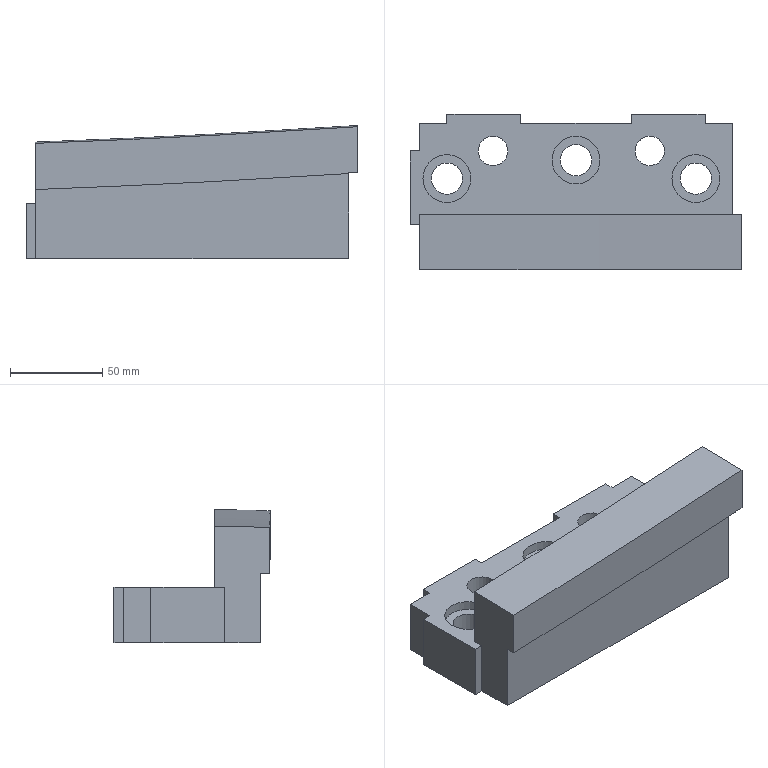Part | NX | features solid 2 | 1 solid | 35 faces | box 180 x 84.614 x 72.162 mm | volume 542810 mm3 | plane 22 | cylinder 8 | spline 5 | commonest cylinder face diameters 17 x3 26 x3 16 x2
STEP:
#1=CARTESIAN_POINT('',(526.5,240.,-40.));
#2=VERTEX_POINT('',#1);
#3=CARTESIAN_POINT('',(535.,240.,-40.));
#4=DIRECTION('',(0.,0.,-1.));
#5=DIRECTION('',(-1.,0.,0.));
#6=AXIS2_PLACEMENT_3D('',#3,#4,#5);
#7=CIRCLE('',#6,8.5);
#8=EDGE_CURVE('',#2,#2,#7,.T.);
#9=ORIENTED_EDGE('',*,*,#8,.F.);
#10=EDGE_LOOP('',(#9));
#11=FACE_BOUND('',#10,.T.);
#12=CARTESIAN_POINT('',(461.5,250.,-40.));
#13=VERTEX_POINT('',#12);
#14=CARTESIAN_POINT('',(470.,250.,-40.));
#15=DIRECTION('',(0.,0.,-1.));
#16=DIRECTION('',(-1.,0.,0.));
#17=AXIS2_PLACEMENT_3D('',#14,#15,#16);
#18=CIRCLE('',#17,8.5);
#19=EDGE_CURVE('',#13,#13,#18,.T.);
#20=ORIENTED_EDGE('',*,*,#19,.F.);
#21=EDGE_LOOP('',(#20));
#22=FACE_BOUND('',#21,.T.);
#23=CARTESIAN_POINT('',(391.5,240.,-40.));
#24=VERTEX_POINT('',#23);
#25=CARTESIAN_POINT('',(400.,240.,-40.));
#26=DIRECTION('',(0.,0.,-1.));
#27=DIRECTION('',(-1.,0.,0.));
#28=AXIS2_PLACEMENT_3D('',#25,#26,#27);
#29=CIRCLE('',#28,8.5);
#30=EDGE_CURVE('',#24,#24,#29,.T.);
#31=ORIENTED_EDGE('',*,*,#30,.F.);
#32=EDGE_LOOP('',(#31));
#33=FACE_BOUND('',#32,.T.);
#34=CARTESIAN_POINT('',(502.,255.,-40.));
#35=VERTEX_POINT('',#34);
#36=CARTESIAN_POINT('',(510.,255.,-40.));
#37=DIRECTION('',(0.,0.,-1.));
#38=DIRECTION('',(-1.,0.,0.));
#39=AXIS2_PLACEMENT_3D('',#36,#37,#38);
#40=CIRCLE('',#39,8.);
#41=EDGE_CURVE('',#35,#35,#40,.F.);
#42=ORIENTED_EDGE('',*,*,#41,.T.);
#43=EDGE_LOOP('',(#42));
#44=FACE_BOUND('',#43,.T.);
#45=CARTESIAN_POINT('',(385.,270.,-40.));
#46=VERTEX_POINT('',#45);
#47=CARTESIAN_POINT('',(385.,255.,-40.));
#48=VERTEX_POINT('',#47);
#49=CARTESIAN_POINT('',(385.,62.718,-40.));
#50=DIRECTION('',(0.,-1.,0.));
#51=VECTOR('',#50,1000.);
#52=LINE('',#49,#51);
#53=EDGE_CURVE('',#46,#48,#52,.T.);
#54=ORIENTED_EDGE('',*,*,#53,.F.);
#55=CARTESIAN_POINT('',(400.,270.,-40.));
#56=VERTEX_POINT('',#55);
#57=CARTESIAN_POINT('',(660.,270.,-40.));
#58=DIRECTION('',(1.,0.,0.));
#59=VECTOR('',#58,1000.);
#60=LINE('',#57,#59);
#61=EDGE_CURVE('',#56,#46,#60,.F.);
#62=ORIENTED_EDGE('',*,*,#61,.F.);
#63=CARTESIAN_POINT('',(400.,275.,-40.));
#64=VERTEX_POINT('',#63);
#65=CARTESIAN_POINT('',(400.,270.,-40.));
#66=DIRECTION('',(0.,-1.,0.));
#67=VECTOR('',#66,1000.);
#68=LINE('',#65,#67);
#69=EDGE_CURVE('',#56,#64,#68,.F.);
#70=ORIENTED_EDGE('',*,*,#69,.T.);
#71=CARTESIAN_POINT('',(440.,275.,-40.));
#72=VERTEX_POINT('',#71);
#73=CARTESIAN_POINT('',(440.,275.,-40.));
#74=DIRECTION('',(1.,0.,0.));
#75=VECTOR('',#74,1000.);
#76=LINE('',#73,#75);
#77=EDGE_CURVE('',#72,#64,#76,.F.);
#78=ORIENTED_EDGE('',*,*,#77,.F.);
#79=CARTESIAN_POINT('',(440.,270.,-40.));
#80=VERTEX_POINT('',#79);
#81=CARTESIAN_POINT('',(440.,270.,-40.));
#82=DIRECTION('',(0.,-1.,0.));
#83=VECTOR('',#82,1000.);
#84=LINE('',#81,#83);
#85=EDGE_CURVE('',#80,#72,#84,.F.);
#86=ORIENTED_EDGE('',*,*,#85,.F.);
#87=CARTESIAN_POINT('',(500.,270.,-40.));
#88=VERTEX_POINT('',#87);
#89=CARTESIAN_POINT('',(660.,270.,-40.));
#90=DIRECTION('',(1.,0.,0.));
#91=VECTOR('',#90,1000.);
#92=LINE('',#89,#91);
#93=EDGE_CURVE('',#88,#80,#92,.F.);
#94=ORIENTED_EDGE('',*,*,#93,.F.);
#95=CARTESIAN_POINT('',(500.,275.,-40.));
#96=VERTEX_POINT('',#95);
#97=CARTESIAN_POINT('',(500.,270.,-40.));
#98=DIRECTION('',(0.,-1.,0.));
#99=VECTOR('',#98,1000.);
#100=LINE('',#97,#99);
#101=EDGE_CURVE('',#88,#96,#100,.F.);
#102=ORIENTED_EDGE('',*,*,#101,.T.);
#103=CARTESIAN_POINT('',(540.,275.,-40.));
#104=VERTEX_POINT('',#103);
#105=CARTESIAN_POINT('',(540.,275.,-40.));
#106=DIRECTION('',(1.,0.,0.));
#107=VECTOR('',#106,1000.);
#108=LINE('',#105,#107);
#109=EDGE_CURVE('',#104,#96,#108,.F.);
#110=ORIENTED_EDGE('',*,*,#109,.F.);
#111=CARTESIAN_POINT('',(540.,270.,-40.));
#112=VERTEX_POINT('',#111);
#113=CARTESIAN_POINT('',(540.,270.,-40.));
#114=DIRECTION('',(0.,-1.,0.));
#115=VECTOR('',#114,1000.);
#116=LINE('',#113,#115);
#117=EDGE_CURVE('',#112,#104,#116,.F.);
#118=ORIENTED_EDGE('',*,*,#117,.F.);
#119=CARTESIAN_POINT('',(555.,270.,-40.));
#120=VERTEX_POINT('',#119);
#121=CARTESIAN_POINT('',(660.,270.,-40.));
#122=DIRECTION('',(1.,0.,0.));
#123=VECTOR('',#122,1000.);
#124=LINE('',#121,#123);
#125=EDGE_CURVE('',#120,#112,#124,.F.);
#126=ORIENTED_EDGE('',*,*,#125,.F.);
#127=CARTESIAN_POINT('',(555.,195.38,-40.));
#128=VERTEX_POINT('',#127);
#129=CARTESIAN_POINT('',(555.,62.718,-40.));
#130=DIRECTION('',(0.,1.,0.));
#131=VECTOR('',#130,1000.);
#132=LINE('',#129,#131);
#133=EDGE_CURVE('',#128,#120,#132,.T.);
#134=ORIENTED_EDGE('',*,*,#133,.F.);
#135=CARTESIAN_POINT('',(385.,195.487,-40.));
#136=VERTEX_POINT('',#135);
#137=CARTESIAN_POINT('',(385.,195.487,-40.));
#138=CARTESIAN_POINT('',(413.333,195.462,-40.));
#139=CARTESIAN_POINT('',(470.,195.441,-40.));
#140=CARTESIAN_POINT('',(526.667,195.352,-40.));
#141=CARTESIAN_POINT('',(555.,195.38,-40.));
#142=B_SPLINE_CURVE_WITH_KNOTS('',3,(#137,#138,#139,#140,#141),.UNSPECIFIED.,.F.,.F.,(4,1,4),(0.1223,0.2065,0.2908),.UNSPECIFIED.);
#143=EDGE_CURVE('',#136,#128,#142,.T.);
#144=ORIENTED_EDGE('',*,*,#143,.F.);
#145=CARTESIAN_POINT('',(385.,215.,-40.));
#146=VERTEX_POINT('',#145);
#147=CARTESIAN_POINT('',(385.,62.718,-40.));
#148=DIRECTION('',(0.,-1.,0.));
#149=VECTOR('',#148,1000.);
#150=LINE('',#147,#149);
#151=EDGE_CURVE('',#146,#136,#150,.T.);
#152=ORIENTED_EDGE('',*,*,#151,.F.);
#153=CARTESIAN_POINT('',(380.,215.,-40.));
#154=VERTEX_POINT('',#153);
#155=CARTESIAN_POINT('',(385.,215.,-40.));
#156=DIRECTION('',(1.,0.,0.));
#157=VECTOR('',#156,1000.);
#158=LINE('',#155,#157);
#159=EDGE_CURVE('',#146,#154,#158,.F.);
#160=ORIENTED_EDGE('',*,*,#159,.T.);
#161=CARTESIAN_POINT('',(380.,255.,-40.));
#162=VERTEX_POINT('',#161);
#163=CARTESIAN_POINT('',(380.,270.,-40.));
#164=DIRECTION('',(0.,1.,0.));
#165=VECTOR('',#164,1000.);
#166=LINE('',#163,#165);
#167=EDGE_CURVE('',#154,#162,#166,.T.);
#168=ORIENTED_EDGE('',*,*,#167,.T.);
#169=CARTESIAN_POINT('',(385.,255.,-40.));
#170=DIRECTION('',(1.,0.,0.));
#171=VECTOR('',#170,1000.);
#172=LINE('',#169,#171);
#173=EDGE_CURVE('',#48,#162,#172,.F.);
#174=ORIENTED_EDGE('',*,*,#173,.F.);
#175=EDGE_LOOP('',(#54,#62,#70,#78,#86,#94,#102,#110,#118,#126,#134,#144,#152,#160,#168,#174));
#176=FACE_BOUND('',#175,.T.);
#177=CARTESIAN_POINT('',(417.,255.,-40.));
#178=VERTEX_POINT('',#177);
#179=CARTESIAN_POINT('',(425.,255.,-40.));
#180=DIRECTION('',(0.,0.,-1.));
#181=DIRECTION('',(-1.,0.,0.));
#182=AXIS2_PLACEMENT_3D('',#179,#180,#181);
#183=CIRCLE('',#182,8.);
#184=EDGE_CURVE('',#178,#178,#183,.F.);
#185=ORIENTED_EDGE('',*,*,#184,.T.);
#186=EDGE_LOOP('',(#185));
#187=FACE_BOUND('',#186,.T.);
#188=CARTESIAN_POINT('',(248.595,62.718,-40.));
#189=DIRECTION('',(0.,0.,-1.));
#190=DIRECTION('',(1.,0.,0.));
#191=AXIS2_PLACEMENT_3D('',#188,#189,#190);
#192=PLANE('',#191);
#193=ADVANCED_FACE('',(#11,#22,#33,#44,#176,#187),#192,.T.);
#194=CARTESIAN_POINT('',(522.,240.,-10.));
#195=VERTEX_POINT('',#194);
#196=CARTESIAN_POINT('',(535.,240.,-10.));
#197=DIRECTION('',(0.,0.,-1.));
#198=DIRECTION('',(-1.,0.,0.));
#199=AXIS2_PLACEMENT_3D('',#196,#197,#198);
#200=CIRCLE('',#199,13.);
#201=EDGE_CURVE('',#195,#195,#200,.T.);
#202=ORIENTED_EDGE('',*,*,#201,.T.);
#203=EDGE_LOOP('',(#202));
#204=FACE_BOUND('',#203,.T.);
#205=CARTESIAN_POINT('',(457.,250.,-10.));
#206=VERTEX_POINT('',#205);
#207=CARTESIAN_POINT('',(470.,250.,-10.));
#208=DIRECTION('',(0.,0.,-1.));
#209=DIRECTION('',(-1.,0.,0.));
#210=AXIS2_PLACEMENT_3D('',#207,#208,#209);
#211=CIRCLE('',#210,13.);
#212=EDGE_CURVE('',#206,#206,#211,.T.);
#213=ORIENTED_EDGE('',*,*,#212,.T.);
#214=EDGE_LOOP('',(#213));
#215=FACE_BOUND('',#214,.T.);
#216=CARTESIAN_POINT('',(387.,240.,-10.));
#217=VERTEX_POINT('',#216);
#218=CARTESIAN_POINT('',(400.,240.,-10.));
#219=DIRECTION('',(0.,0.,-1.));
#220=DIRECTION('',(-1.,0.,0.));
#221=AXIS2_PLACEMENT_3D('',#218,#219,#220);
#222=CIRCLE('',#221,13.);
#223=EDGE_CURVE('',#217,#217,#222,.T.);
#224=ORIENTED_EDGE('',*,*,#223,.T.);
#225=EDGE_LOOP('',(#224));
#226=FACE_BOUND('',#225,.T.);
#227=CARTESIAN_POINT('',(502.,255.,-10.));
#228=VERTEX_POINT('',#227);
#229=CARTESIAN_POINT('',(510.,255.,-10.));
#230=DIRECTION('',(0.,0.,-1.));
#231=DIRECTION('',(-1.,0.,0.));
#232=AXIS2_PLACEMENT_3D('',#229,#230,#231);
#233=CIRCLE('',#232,8.);
#234=EDGE_CURVE('',#228,#228,#233,.F.);
#235=ORIENTED_EDGE('',*,*,#234,.F.);
#236=EDGE_LOOP('',(#235));
#237=FACE_BOUND('',#236,.T.);
#238=CARTESIAN_POINT('',(555.,270.,-10.));
#239=VERTEX_POINT('',#238);
#240=CARTESIAN_POINT('',(540.,270.,-10.));
#241=VERTEX_POINT('',#240);
#242=CARTESIAN_POINT('',(660.,270.,-10.));
#243=DIRECTION('',(-1.,0.,0.));
#244=VECTOR('',#243,1000.);
#245=LINE('',#242,#244);
#246=EDGE_CURVE('',#239,#241,#245,.T.);
#247=ORIENTED_EDGE('',*,*,#246,.T.);
#248=CARTESIAN_POINT('',(540.,275.,-10.));
#249=VERTEX_POINT('',#248);
#250=CARTESIAN_POINT('',(540.,270.,-10.));
#251=DIRECTION('',(0.,-1.,0.));
#252=VECTOR('',#251,1000.);
#253=LINE('',#250,#252);
#254=EDGE_CURVE('',#241,#249,#253,.F.);
#255=ORIENTED_EDGE('',*,*,#254,.T.);
#256=CARTESIAN_POINT('',(500.,275.,-10.));
#257=VERTEX_POINT('',#256);
#258=CARTESIAN_POINT('',(540.,275.,-10.));
#259=DIRECTION('',(1.,0.,0.));
#260=VECTOR('',#259,1000.);
#261=LINE('',#258,#260);
#262=EDGE_CURVE('',#249,#257,#261,.F.);
#263=ORIENTED_EDGE('',*,*,#262,.T.);
#264=CARTESIAN_POINT('',(500.,270.,-10.));
#265=VERTEX_POINT('',#264);
#266=CARTESIAN_POINT('',(500.,270.,-10.));
#267=DIRECTION('',(0.,-1.,0.));
#268=VECTOR('',#267,1000.);
#269=LINE('',#266,#268);
#270=EDGE_CURVE('',#265,#257,#269,.F.);
#271=ORIENTED_EDGE('',*,*,#270,.F.);
#272=CARTESIAN_POINT('',(440.,270.,-10.));
#273=VERTEX_POINT('',#272);
#274=CARTESIAN_POINT('',(660.,270.,-10.));
#275=DIRECTION('',(-1.,0.,0.));
#276=VECTOR('',#275,1000.);
#277=LINE('',#274,#276);
#278=EDGE_CURVE('',#265,#273,#277,.T.);
#279=ORIENTED_EDGE('',*,*,#278,.T.);
#280=CARTESIAN_POINT('',(440.,275.,-10.));
#281=VERTEX_POINT('',#280);
#282=CARTESIAN_POINT('',(440.,270.,-10.));
#283=DIRECTION('',(0.,-1.,0.));
#284=VECTOR('',#283,1000.);
#285=LINE('',#282,#284);
#286=EDGE_CURVE('',#273,#281,#285,.F.);
#287=ORIENTED_EDGE('',*,*,#286,.T.);
#288=CARTESIAN_POINT('',(400.,275.,-10.));
#289=VERTEX_POINT('',#288);
#290=CARTESIAN_POINT('',(440.,275.,-10.));
#291=DIRECTION('',(1.,0.,0.));
#292=VECTOR('',#291,1000.);
#293=LINE('',#290,#292);
#294=EDGE_CURVE('',#281,#289,#293,.F.);
#295=ORIENTED_EDGE('',*,*,#294,.T.);
#296=CARTESIAN_POINT('',(400.,270.,-10.));
#297=VERTEX_POINT('',#296);
#298=CARTESIAN_POINT('',(400.,270.,-10.));
#299=DIRECTION('',(0.,-1.,0.));
#300=VECTOR('',#299,1000.);
#301=LINE('',#298,#300);
#302=EDGE_CURVE('',#297,#289,#301,.F.);
#303=ORIENTED_EDGE('',*,*,#302,.F.);
#304=CARTESIAN_POINT('',(385.,270.,-10.));
#305=VERTEX_POINT('',#304);
#306=CARTESIAN_POINT('',(660.,270.,-10.));
#307=DIRECTION('',(-1.,0.,0.));
#308=VECTOR('',#307,1000.);
#309=LINE('',#306,#308);
#310=EDGE_CURVE('',#297,#305,#309,.T.);
#311=ORIENTED_EDGE('',*,*,#310,.T.);
#312=CARTESIAN_POINT('',(385.,255.,-10.));
#313=VERTEX_POINT('',#312);
#314=CARTESIAN_POINT('',(385.,270.,-10.));
#315=DIRECTION('',(0.,-1.,0.));
#316=VECTOR('',#315,1000.);
#317=LINE('',#314,#316);
#318=EDGE_CURVE('',#305,#313,#317,.T.);
#319=ORIENTED_EDGE('',*,*,#318,.T.);
#320=CARTESIAN_POINT('',(380.,255.,-10.));
#321=VERTEX_POINT('',#320);
#322=CARTESIAN_POINT('',(385.,255.,-10.));
#323=DIRECTION('',(1.,0.,0.));
#324=VECTOR('',#323,1000.);
#325=LINE('',#322,#324);
#326=EDGE_CURVE('',#313,#321,#325,.F.);
#327=ORIENTED_EDGE('',*,*,#326,.T.);
#328=CARTESIAN_POINT('',(380.,215.,-10.));
#329=VERTEX_POINT('',#328);
#330=CARTESIAN_POINT('',(380.,270.,-10.));
#331=DIRECTION('',(0.,1.,0.));
#332=VECTOR('',#331,1000.);
#333=LINE('',#330,#332);
#334=EDGE_CURVE('',#329,#321,#333,.T.);
#335=ORIENTED_EDGE('',*,*,#334,.F.);
#336=CARTESIAN_POINT('',(385.,215.,-10.));
#337=VERTEX_POINT('',#336);
#338=CARTESIAN_POINT('',(385.,215.,-10.));
#339=DIRECTION('',(1.,0.,0.));
#340=VECTOR('',#339,1000.);
#341=LINE('',#338,#340);
#342=EDGE_CURVE('',#337,#329,#341,.F.);
#343=ORIENTED_EDGE('',*,*,#342,.F.);
#344=CARTESIAN_POINT('',(385.,220.484,-10.));
#345=VERTEX_POINT('',#344);
#346=CARTESIAN_POINT('',(385.,270.,-10.));
#347=DIRECTION('',(0.,1.,0.));
#348=VECTOR('',#347,1000.);
#349=LINE('',#346,#348);
#350=EDGE_CURVE('',#337,#345,#349,.T.);
#351=ORIENTED_EDGE('',*,*,#350,.T.);
#352=CARTESIAN_POINT('',(555.,220.387,-10.));
#353=VERTEX_POINT('',#352);
#354=CARTESIAN_POINT('',(560.,220.386,-10.));
#355=CARTESIAN_POINT('',(526.442,220.392,-10.));
#356=CARTESIAN_POINT('',(476.105,220.419,-10.));
#357=CARTESIAN_POINT('',(408.97,220.463,-10.));
#358=CARTESIAN_POINT('',(366.895,220.496,-10.));
#359=CARTESIAN_POINT('',(333.741,220.565,-10.));
#360=CARTESIAN_POINT('',(314.827,220.599,-10.));
#361=CARTESIAN_POINT('',(301.695,220.599,-10.));
#362=CARTESIAN_POINT('',(297.997,220.637,-10.));
#363=CARTESIAN_POINT('',(290.161,220.611,-10.));
#364=CARTESIAN_POINT('',(281.479,219.228,-10.));
#365=CARTESIAN_POINT('',(272.181,215.568,-10.));
#366=CARTESIAN_POINT('',(264.352,210.189,-10.));
#367=CARTESIAN_POINT('',(257.821,203.431,-10.));
#368=CARTESIAN_POINT('',(253.634,196.762,-10.));
#369=CARTESIAN_POINT('',(251.086,190.582,-10.));
#370=CARTESIAN_POINT('',(249.212,184.171,-10.));
#371=CARTESIAN_POINT('',(248.528,177.262,-10.));
#372=CARTESIAN_POINT('',(248.548,172.265,-10.));
#373=CARTESIAN_POINT('',(248.587,169.669,-10.));
#374=CARTESIAN_POINT('',(248.59,166.626,-10.));
#375=CARTESIAN_POINT('',(248.575,155.998,-10.));
#376=CARTESIAN_POINT('',(248.59,138.236,-10.));
#377=CARTESIAN_POINT('',(248.599,104.71,-10.));
#378=CARTESIAN_POINT('',(248.592,45.941,-10.));
#379=CARTESIAN_POINT('',(248.598,-12.772,-10.));
#380=CARTESIAN_POINT('',(248.605,-63.152,-10.));
#381=CARTESIAN_POINT('',(248.59,-84.03,-10.));
#382=CARTESIAN_POINT('',(248.581,-100.973,-10.));
#383=CARTESIAN_POINT('',(248.614,-110.39,-10.));
#384=CARTESIAN_POINT('',(248.565,-116.228,-10.));
#385=CARTESIAN_POINT('',(248.487,-119.918,-10.));
#386=CARTESIAN_POINT('',(248.926,-126.9,-10.));
#387=CARTESIAN_POINT('',(250.444,-133.072,-10.));
#388=CARTESIAN_POINT('',(252.598,-139.093,-10.));
#389=CARTESIAN_POINT('',(256.391,-145.942,-10.));
#390=CARTESIAN_POINT('',(262.559,-153.127,-10.));
#391=CARTESIAN_POINT('',(270.075,-158.887,-10.));
#392=CARTESIAN_POINT('',(277.474,-162.344,-10.));
#393=CARTESIAN_POINT('',(283.712,-164.068,-10.));
#394=CARTESIAN_POINT('',(289.455,-165.043,-10.));
#395=CARTESIAN_POINT('',(297.812,-165.183,-10.));
#396=CARTESIAN_POINT('',(302.108,-165.054,-10.));
#397=CARTESIAN_POINT('',(318.79,-165.12,-10.));
#398=CARTESIAN_POINT('',(346.789,-165.069,-10.));
#399=CARTESIAN_POINT('',(406.469,-165.113,-10.));
#400=CARTESIAN_POINT('',(456.436,-165.108,-10.));
#401=CARTESIAN_POINT('',(490.,-165.147,-10.));
#402=B_SPLINE_CURVE_WITH_KNOTS('',3,(#354,#355,#356,#357,#358,#359,#360,#361,#362,#363,#364,#365,#366,#367,#368,#369,#370,#371,#372,#373,#374,#375,#376,#377,#378,#379,#380,#381,#382,#383,#384,#385,#386,#387,#388,#389,#390,#391,#392,#393,#394,#395,#396,#397,#398,#399,#400,#401),.UNSPECIFIED.,.F.,.F.,(4,1,1,1,1,1,1,1,1,1,1,1,1,1,1,1,1,1,1,1,1,1,1,1,1,1,1,1,1,1,1,1,1,1,1,1,1,1,1,1,1,1,1,1,1,4),(0.,0.125,0.1875,0.25,0.2812,0.3125,0.3203,0.3281,0.332,0.3359,0.3398,0.3437,0.3476,0.3515,0.3535,0.3554,0.3594,0.3633,0.3672,0.3711,0.375,0.4062,0.4375,0.5,0.625,0.6562,0.6875,0.7031,0.7187,0.7226,0.7265,0.7304,0.7324,0.7343,0.7382,0.7422,0.7461,0.75,0.7519,0.7539,0.7578,0.7656,0.7812,0.8125,0.875,1.),.UNSPECIFIED.);
#403=EDGE_CURVE('',#353,#345,#402,.T.);
#404=ORIENTED_EDGE('',*,*,#403,.F.);
#405=CARTESIAN_POINT('',(555.,270.,-10.));
#406=DIRECTION('',(0.,1.,0.));
#407=VECTOR('',#406,1000.);
#408=LINE('',#405,#407);
#409=EDGE_CURVE('',#353,#239,#408,.T.);
#410=ORIENTED_EDGE('',*,*,#409,.T.);
#411=EDGE_LOOP('',(#247,#255,#263,#271,#279,#287,#295,#303,#311,#319,#327,#335,#343,#351,#404,#410));
#412=FACE_BOUND('',#411,.T.);
#413=CARTESIAN_POINT('',(417.,255.,-10.));
#414=VERTEX_POINT('',#413);
#415=CARTESIAN_POINT('',(425.,255.,-10.));
#416=DIRECTION('',(0.,0.,-1.));
#417=DIRECTION('',(-1.,0.,0.));
#418=AXIS2_PLACEMENT_3D('',#415,#416,#417);
#419=CIRCLE('',#418,8.);
#420=EDGE_CURVE('',#414,#414,#419,.F.);
#421=ORIENTED_EDGE('',*,*,#420,.F.);
#422=EDGE_LOOP('',(#421));
#423=FACE_BOUND('',#422,.T.);
#424=CARTESIAN_POINT('',(660.,270.,-10.));
#425=DIRECTION('',(0.,0.,-1.));
#426=DIRECTION('',(1.,0.,0.));
#427=AXIS2_PLACEMENT_3D('',#424,#425,#426);
#428=PLANE('',#427);
#429=ADVANCED_FACE('',(#204,#215,#226,#237,#412,#423),#428,.F.);
#430=CARTESIAN_POINT('',(385.,255.,-40.));
#431=DIRECTION('',(0.,0.,-1.));
#432=VECTOR('',#431,1000.);
#433=LINE('',#430,#432);
#434=EDGE_CURVE('',#48,#313,#433,.F.);
#435=ORIENTED_EDGE('',*,*,#434,.T.);
#436=ORIENTED_EDGE('',*,*,#318,.F.);
#437=CARTESIAN_POINT('',(385.,270.,-10.));
#438=DIRECTION('',(0.,0.,-1.));
#439=VECTOR('',#438,1000.);
#440=LINE('',#437,#439);
#441=EDGE_CURVE('',#46,#305,#440,.F.);
#442=ORIENTED_EDGE('',*,*,#441,.F.);
#443=ORIENTED_EDGE('',*,*,#53,.T.);
#444=EDGE_LOOP('',(#435,#436,#442,#443));
#445=FACE_BOUND('',#444,.T.);
#446=CARTESIAN_POINT('',(385.,-1383.009,0.));
#447=DIRECTION('',(1.,0.,0.));
#448=DIRECTION('',(0.,0.,-1.));
#449=AXIS2_PLACEMENT_3D('',#446,#447,#448);
#450=PLANE('',#449);
#451=ADVANCED_FACE('',(#445),#450,.F.);
#452=CARTESIAN_POINT('',(440.,270.,-10.));
#453=DIRECTION('',(0.,0.,-1.));
#454=VECTOR('',#453,1000.);
#455=LINE('',#452,#454);
#456=EDGE_CURVE('',#273,#80,#455,.T.);
#457=ORIENTED_EDGE('',*,*,#456,.F.);
#458=ORIENTED_EDGE('',*,*,#278,.F.);
#459=CARTESIAN_POINT('',(500.,270.,-10.));
#460=DIRECTION('',(0.,0.,-1.));
#461=VECTOR('',#460,1000.);
#462=LINE('',#459,#461);
#463=EDGE_CURVE('',#265,#88,#462,.T.);
#464=ORIENTED_EDGE('',*,*,#463,.T.);
#465=ORIENTED_EDGE('',*,*,#93,.T.);
#466=EDGE_LOOP('',(#457,#458,#464,#465));
#467=FACE_BOUND('',#466,.T.);
#468=CARTESIAN_POINT('',(660.,270.,-10.));
#469=DIRECTION('',(0.,1.,0.));
#470=DIRECTION('',(-1.,0.,0.));
#471=AXIS2_PLACEMENT_3D('',#468,#469,#470);
#472=PLANE('',#471);
#473=ADVANCED_FACE('',(#467),#472,.T.);
#474=CARTESIAN_POINT('',(400.,270.,-10.));
#475=DIRECTION('',(0.,0.,-1.));
#476=VECTOR('',#475,1000.);
#477=LINE('',#474,#476);
#478=EDGE_CURVE('',#297,#56,#477,.T.);
#479=ORIENTED_EDGE('',*,*,#478,.T.);
#480=ORIENTED_EDGE('',*,*,#61,.T.);
#481=ORIENTED_EDGE('',*,*,#441,.T.);
#482=ORIENTED_EDGE('',*,*,#310,.F.);
#483=EDGE_LOOP('',(#479,#480,#481,#482));
#484=FACE_BOUND('',#483,.T.);
#485=CARTESIAN_POINT('',(660.,270.,-10.));
#486=DIRECTION('',(0.,1.,0.));
#487=DIRECTION('',(-1.,0.,0.));
#488=AXIS2_PLACEMENT_3D('',#485,#486,#487);
#489=PLANE('',#488);
#490=ADVANCED_FACE('',(#484),#489,.T.);
#491=CARTESIAN_POINT('',(540.,270.,-10.));
#492=DIRECTION('',(0.,0.,-1.));
#493=VECTOR('',#492,1000.);
#494=LINE('',#491,#493);
#495=EDGE_CURVE('',#241,#112,#494,.T.);
#496=ORIENTED_EDGE('',*,*,#495,.F.);
#497=ORIENTED_EDGE('',*,*,#246,.F.);
#498=CARTESIAN_POINT('',(555.,270.,6.411));
#499=DIRECTION('',(0.,0.,-1.));
#500=VECTOR('',#499,1000.);
#501=LINE('',#498,#500);
#502=EDGE_CURVE('',#239,#120,#501,.T.);
#503=ORIENTED_EDGE('',*,*,#502,.T.);
#504=ORIENTED_EDGE('',*,*,#125,.T.);
#505=EDGE_LOOP('',(#496,#497,#503,#504));
#506=FACE_BOUND('',#505,.T.);
#507=CARTESIAN_POINT('',(660.,270.,-10.));
#508=DIRECTION('',(0.,1.,0.));
#509=DIRECTION('',(-1.,0.,0.));
#510=AXIS2_PLACEMENT_3D('',#507,#508,#509);
#511=PLANE('',#510);
#512=ADVANCED_FACE('',(#506),#511,.T.);
#513=ORIENTED_EDGE('',*,*,#403,.T.);
#514=CARTESIAN_POINT('',(385.,220.484,23.155));
#515=VERTEX_POINT('',#514);
#516=CARTESIAN_POINT('',(385.,220.484,6.67));
#517=DIRECTION('',(0.,0.,1.));
#518=VECTOR('',#517,1000.);
#519=LINE('',#516,#518);
#520=EDGE_CURVE('',#345,#515,#519,.T.);
#521=ORIENTED_EDGE('',*,*,#520,.T.);
#522=CARTESIAN_POINT('',(560.,220.386,32.162));
#523=VERTEX_POINT('',#522);
#524=CARTESIAN_POINT('',(560.,220.386,32.162));
#525=CARTESIAN_POINT('',(501.705,220.396,28.304));
#526=CARTESIAN_POINT('',(443.371,220.428,25.302));
#527=CARTESIAN_POINT('',(385.,220.484,23.155));
#528=B_SPLINE_CURVE_WITH_KNOTS('',3,(#524,#525,#526,#527),.UNSPECIFIED.,.F.,.F.,(4,4),(0.,0.1752),.UNSPECIFIED.);
#529=EDGE_CURVE('',#523,#515,#528,.T.);
#530=ORIENTED_EDGE('',*,*,#529,.F.);
#531=CARTESIAN_POINT('',(560.,220.386,6.411));
#532=VERTEX_POINT('',#531);
#533=CARTESIAN_POINT('',(560.,220.386,-300.));
#534=DIRECTION('',(0.,0.,1.));
#535=VECTOR('',#534,1000.);
#536=LINE('',#533,#535);
#537=EDGE_CURVE('',#532,#523,#536,.T.);
#538=ORIENTED_EDGE('',*,*,#537,.F.);
#539=CARTESIAN_POINT('',(555.,220.387,6.411));
#540=VERTEX_POINT('',#539);
#541=CARTESIAN_POINT('',(560.,220.386,6.411));
#542=CARTESIAN_POINT('',(526.442,220.392,6.411));
#543=CARTESIAN_POINT('',(476.105,220.419,6.411));
#544=CARTESIAN_POINT('',(408.97,220.463,6.411));
#545=CARTESIAN_POINT('',(366.895,220.496,6.411));
#546=CARTESIAN_POINT('',(333.741,220.565,6.411));
#547=CARTESIAN_POINT('',(314.827,220.599,6.411));
#548=CARTESIAN_POINT('',(301.695,220.599,6.411));
#549=CARTESIAN_POINT('',(297.997,220.637,6.411));
#550=CARTESIAN_POINT('',(290.161,220.611,6.411));
#551=CARTESIAN_POINT('',(281.479,219.228,6.411));
#552=CARTESIAN_POINT('',(272.181,215.568,6.411));
#553=CARTESIAN_POINT('',(264.352,210.189,6.411));
#554=CARTESIAN_POINT('',(257.821,203.431,6.411));
#555=CARTESIAN_POINT('',(253.634,196.762,6.411));
#556=CARTESIAN_POINT('',(251.086,190.582,6.411));
#557=CARTESIAN_POINT('',(249.212,184.171,6.411));
#558=CARTESIAN_POINT('',(248.528,177.262,6.411));
#559=CARTESIAN_POINT('',(248.548,172.265,6.411));
#560=CARTESIAN_POINT('',(248.587,169.669,6.411));
#561=CARTESIAN_POINT('',(248.59,166.626,6.411));
#562=CARTESIAN_POINT('',(248.575,155.998,6.411));
#563=CARTESIAN_POINT('',(248.59,138.236,6.411));
#564=CARTESIAN_POINT('',(248.599,104.71,6.411));
#565=CARTESIAN_POINT('',(248.592,45.941,6.411));
#566=CARTESIAN_POINT('',(248.598,-12.772,6.411));
#567=CARTESIAN_POINT('',(248.605,-63.152,6.411));
#568=CARTESIAN_POINT('',(248.59,-84.03,6.411));
#569=CARTESIAN_POINT('',(248.581,-100.973,6.411));
#570=CARTESIAN_POINT('',(248.614,-110.39,6.411));
#571=CARTESIAN_POINT('',(248.565,-116.228,6.411));
#572=CARTESIAN_POINT('',(248.487,-119.918,6.411));
#573=CARTESIAN_POINT('',(248.926,-126.9,6.411));
#574=CARTESIAN_POINT('',(250.444,-133.072,6.411));
#575=CARTESIAN_POINT('',(252.598,-139.093,6.411));
#576=CARTESIAN_POINT('',(256.391,-145.942,6.411));
#577=CARTESIAN_POINT('',(262.559,-153.127,6.411));
#578=CARTESIAN_POINT('',(270.075,-158.887,6.411));
#579=CARTESIAN_POINT('',(277.474,-162.344,6.411));
#580=CARTESIAN_POINT('',(283.712,-164.068,6.411));
#581=CARTESIAN_POINT('',(289.455,-165.043,6.411));
#582=CARTESIAN_POINT('',(297.812,-165.183,6.411));
#583=CARTESIAN_POINT('',(302.108,-165.054,6.411));
#584=CARTESIAN_POINT('',(318.79,-165.12,6.411));
#585=CARTESIAN_POINT('',(346.789,-165.069,6.411));
#586=CARTESIAN_POINT('',(406.469,-165.113,6.411));
#587=CARTESIAN_POINT('',(456.436,-165.108,6.411));
#588=CARTESIAN_POINT('',(490.,-165.147,6.411));
#589=B_SPLINE_CURVE_WITH_KNOTS('',3,(#541,#542,#543,#544,#545,#546,#547,#548,#549,#550,#551,#552,#553,#554,#555,#556,#557,#558,#559,#560,#561,#562,#563,#564,#565,#566,#567,#568,#569,#570,#571,#572,#573,#574,#575,#576,#577,#578,#579,#580,#581,#582,#583,#584,#585,#586,#587,#588),.UNSPECIFIED.,.F.,.F.,(4,1,1,1,1,1,1,1,1,1,1,1,1,1,1,1,1,1,1,1,1,1,1,1,1,1,1,1,1,1,1,1,1,1,1,1,1,1,1,1,1,1,1,1,1,4),(0.,0.125,0.1875,0.25,0.2812,0.3125,0.3203,0.3281,0.332,0.3359,0.3398,0.3437,0.3476,0.3515,0.3535,0.3554,0.3594,0.3633,0.3672,0.3711,0.375,0.4062,0.4375,0.5,0.625,0.6562,0.6875,0.7031,0.7187,0.7226,0.7265,0.7304,0.7324,0.7343,0.7382,0.7422,0.7461,0.75,0.7519,0.7539,0.7578,0.7656,0.7812,0.8125,0.875,1.),.UNSPECIFIED.);
#590=EDGE_CURVE('',#540,#532,#589,.F.);
#591=ORIENTED_EDGE('',*,*,#590,.F.);
#592=CARTESIAN_POINT('',(555.,220.387,11.207));
#593=DIRECTION('',(0.,0.,1.));
#594=VECTOR('',#593,1000.);
#595=LINE('',#592,#594);
#596=EDGE_CURVE('',#540,#353,#595,.F.);
#597=ORIENTED_EDGE('',*,*,#596,.T.);
#598=EDGE_LOOP('',(#513,#521,#530,#538,#591,#597));
#599=FACE_BOUND('',#598,.T.);
#600=CARTESIAN_POINT('',(560.,220.386,-10.));
#601=CARTESIAN_POINT('',(560.,220.386,32.415));
#602=CARTESIAN_POINT('',(530.845,220.391,-10.));
#603=CARTESIAN_POINT('',(530.845,220.391,32.415));
#604=CARTESIAN_POINT('',(472.562,220.422,-10.));
#605=CARTESIAN_POINT('',(472.562,220.422,32.415));
#606=CARTESIAN_POINT('',(414.164,220.456,-10.));
#607=CARTESIAN_POINT('',(414.164,220.456,32.415));
#608=CARTESIAN_POINT('',(385.,220.484,-10.));
#609=CARTESIAN_POINT('',(385.,220.484,32.415));
#610=B_SPLINE_SURFACE_WITH_KNOTS('',3,1,((#600,#601),(#602,#603),(#604,#605),(#606,#607),(#608,#609)),.SURF_OF_LINEAR_EXTRUSION.,.F.,.F.,.F.,(4,1,4),(2,2),(0.,0.1086,0.2172),(0.,1.),.UNSPECIFIED.);
#611=ADVANCED_FACE('',(#599),#610,.T.);
#612=CARTESIAN_POINT('',(385.,190.489,-2.558));
#613=VERTEX_POINT('',#612);
#614=CARTESIAN_POINT('',(385.,190.489,22.458));
#615=VERTEX_POINT('',#614);
#616=CARTESIAN_POINT('',(385.,190.489,10.136));
#617=DIRECTION('',(0.,0.,1.));
#618=VECTOR('',#617,1000.);
#619=LINE('',#616,#618);
#620=EDGE_CURVE('',#613,#615,#619,.T.);
#621=ORIENTED_EDGE('',*,*,#620,.F.);
#622=CARTESIAN_POINT('',(555.,190.387,6.083));
#623=VERTEX_POINT('',#622);
#624=CARTESIAN_POINT('',(555.,190.387,6.083));
#625=CARTESIAN_POINT('',(498.378,190.399,2.398));
#626=CARTESIAN_POINT('',(441.704,190.437,-0.4813));
#627=CARTESIAN_POINT('',(385.,190.489,-2.558));
#628=B_SPLINE_CURVE_WITH_KNOTS('',3,(#624,#625,#626,#627),.UNSPECIFIED.,.F.,.F.,(4,4),(0.005011,0.1752),.UNSPECIFIED.);
#629=EDGE_CURVE('',#623,#613,#628,.T.);
#630=ORIENTED_EDGE('',*,*,#629,.F.);
#631=CARTESIAN_POINT('',(555.,190.387,6.411));
#632=VERTEX_POINT('',#631);
#633=CARTESIAN_POINT('',(555.,190.387,12.798));
#634=DIRECTION('',(0.,0.,1.));
#635=VECTOR('',#634,1000.);
#636=LINE('',#633,#635);
#637=EDGE_CURVE('',#632,#623,#636,.F.);
#638=ORIENTED_EDGE('',*,*,#637,.F.);
#639=CARTESIAN_POINT('',(560.,190.386,6.411));
#640=VERTEX_POINT('',#639);
#641=CARTESIAN_POINT('',(560.,190.386,6.411));
#642=CARTESIAN_POINT('',(535.789,190.39,6.411));
#643=CARTESIAN_POINT('',(487.367,190.41,6.411));
#644=CARTESIAN_POINT('',(426.839,190.453,6.411));
#645=CARTESIAN_POINT('',(378.417,190.494,6.411));
#646=CARTESIAN_POINT('',(342.103,190.532,6.411));
#647=CARTESIAN_POINT('',(314.858,190.597,6.411));
#648=CARTESIAN_POINT('',(298.223,190.609,6.411));
#649=CARTESIAN_POINT('',(292.157,190.652,6.411));
#650=CARTESIAN_POINT('',(286.192,189.266,6.411));
#651=CARTESIAN_POINT('',(281.366,185.162,6.411));
#652=CARTESIAN_POINT('',(278.872,179.556,6.411));
#653=CARTESIAN_POINT('',(278.5,175.168,6.411));
#654=CARTESIAN_POINT('',(278.587,170.976,6.411));
#655=CARTESIAN_POINT('',(278.584,165.611,6.411));
#656=CARTESIAN_POINT('',(278.586,156.222,6.411));
#657=CARTESIAN_POINT('',(278.595,137.444,6.411));
#658=CARTESIAN_POINT('',(278.596,99.888,6.411));
#659=CARTESIAN_POINT('',(278.593,46.236,6.411));
#660=CARTESIAN_POINT('',(278.601,-7.416,6.411));
#661=CARTESIAN_POINT('',(278.601,-50.338,6.411));
#662=CARTESIAN_POINT('',(278.604,-77.163,6.411));
#663=CARTESIAN_POINT('',(278.577,-95.942,6.411));
#664=CARTESIAN_POINT('',(278.601,-106.672,6.411));
#665=CARTESIAN_POINT('',(278.601,-112.708,6.411));
#666=CARTESIAN_POINT('',(278.556,-116.731,6.411));
#667=CARTESIAN_POINT('',(278.542,-119.416,6.411));
#668=CARTESIAN_POINT('',(278.717,-124.133,6.411));
#669=CARTESIAN_POINT('',(281.719,-130.396,6.411));
#670=CARTESIAN_POINT('',(287.487,-134.298,6.411));
#671=CARTESIAN_POINT('',(292.158,-135.09,6.411));
#672=CARTESIAN_POINT('',(294.84,-135.137,6.411));
#673=CARTESIAN_POINT('',(296.518,-135.111,6.411));
#674=CARTESIAN_POINT('',(307.919,-135.094,6.411));
#675=CARTESIAN_POINT('',(329.38,-135.085,6.411));
#676=CARTESIAN_POINT('',(371.966,-135.101,6.411));
#677=CARTESIAN_POINT('',(425.618,-135.092,6.411));
#678=CARTESIAN_POINT('',(468.539,-135.122,6.411));
#679=CARTESIAN_POINT('',(490.,-135.147,6.411));
#680=B_SPLINE_CURVE_WITH_KNOTS('',3,(#641,#642,#643,#644,#645,#646,#647,#648,#649,#650,#651,#652,#653,#654,#655,#656,#657,#658,#659,#660,#661,#662,#663,#664,#665,#666,#667,#668,#669,#670,#671,#672,#673,#674,#675,#676,#677,#678,#679),.UNSPECIFIED.,.F.,.F.,(4,1,1,1,1,1,1,1,1,1,1,1,1,1,1,1,1,1,1,1,1,1,1,1,1,1,1,1,1,1,1,1,1,1,1,1,4),(0.,0.09016,0.1803,0.2254,0.2705,0.3156,0.3268,0.3325,0.3381,0.3494,0.355,0.3606,0.3656,0.3706,0.3806,0.4006,0.4406,0.5205,0.6004,0.6404,0.6803,0.7003,0.7103,0.7203,0.7228,0.7253,0.7303,0.7403,0.7503,0.7552,0.7577,0.7602,0.7615,0.8002,0.8402,0.9201,1.),.UNSPECIFIED.);
#681=EDGE_CURVE('',#632,#640,#680,.F.);
#682=ORIENTED_EDGE('',*,*,#681,.T.);
#683=CARTESIAN_POINT('',(560.,190.386,31.465));
#684=VERTEX_POINT('',#683);
#685=CARTESIAN_POINT('',(560.,190.386,-300.));
#686=DIRECTION('',(0.,0.,1.));
#687=VECTOR('',#686,1000.);
#688=LINE('',#685,#687);
#689=EDGE_CURVE('',#640,#684,#688,.T.);
#690=ORIENTED_EDGE('',*,*,#689,.T.);
#691=CARTESIAN_POINT('',(560.,190.386,31.465));
#692=CARTESIAN_POINT('',(501.704,190.396,27.608));
#693=CARTESIAN_POINT('',(443.371,190.435,24.606));
#694=CARTESIAN_POINT('',(385.,190.489,22.458));
#695=B_SPLINE_CURVE_WITH_KNOTS('',3,(#691,#692,#693,#694),.UNSPECIFIED.,.F.,.F.,(4,4),(0.,0.1752),.UNSPECIFIED.);
#696=EDGE_CURVE('',#684,#615,#695,.T.);
#697=ORIENTED_EDGE('',*,*,#696,.T.);
#698=EDGE_LOOP('',(#621,#630,#638,#682,#690,#697));
#699=FACE_BOUND('',#698,.T.);
#700=CARTESIAN_POINT('',(560.,190.386,-2.763));
#701=CARTESIAN_POINT('',(560.,190.386,31.67));
#702=CARTESIAN_POINT('',(501.667,190.396,-2.763));
#703=CARTESIAN_POINT('',(501.667,190.396,31.67));
#704=CARTESIAN_POINT('',(443.332,190.435,-2.763));
#705=CARTESIAN_POINT('',(443.332,190.435,31.67));
#706=CARTESIAN_POINT('',(385.,190.489,-2.763));
#707=CARTESIAN_POINT('',(385.,190.489,31.67));
#708=B_SPLINE_SURFACE_WITH_KNOTS('',3,1,((#700,#701),(#702,#703),(#704,#705),(#706,#707)),.SURF_OF_LINEAR_EXTRUSION.,.F.,.F.,.F.,(4,4),(2,2),(0.,0.2172),(0.,1.),.PIECEWISE_BEZIER_KNOTS.);
#709=ADVANCED_FACE('',(#699),#708,.F.);
#710=ORIENTED_EDGE('',*,*,#689,.F.);
#711=CARTESIAN_POINT('',(560.,190.386,6.411));
#712=DIRECTION('',(0.,-1.,0.));
#713=VECTOR('',#712,1000.);
#714=LINE('',#711,#713);
#715=EDGE_CURVE('',#640,#532,#714,.F.);
#716=ORIENTED_EDGE('',*,*,#715,.T.);
#717=ORIENTED_EDGE('',*,*,#537,.T.);
#718=CARTESIAN_POINT('',(560.,190.386,31.465));
#719=CARTESIAN_POINT('',(560.,200.386,31.698));
#720=CARTESIAN_POINT('',(560.,210.386,31.93));
#721=CARTESIAN_POINT('',(560.,220.386,32.162));
#722=B_SPLINE_CURVE_WITH_KNOTS('',3,(#718,#719,#720,#721),.UNSPECIFIED.,.F.,.F.,(4,4),(0.,0.03001),.UNSPECIFIED.);
#723=EDGE_CURVE('',#684,#523,#722,.T.);
#724=ORIENTED_EDGE('',*,*,#723,.F.);
#725=EDGE_LOOP('',(#710,#716,#717,#724));
#726=FACE_BOUND('',#725,.T.);
#727=CARTESIAN_POINT('',(560.,190.386,-300.));
#728=DIRECTION('',(-1.,0.,0.));
#729=DIRECTION('',(0.,0.,-1.));
#730=AXIS2_PLACEMENT_3D('',#727,#728,#729);
#731=PLANE('',#730);
#732=ADVANCED_FACE('',(#726),#731,.F.);
#733=ORIENTED_EDGE('',*,*,#529,.T.);
#734=CARTESIAN_POINT('',(385.,220.484,23.155));
#735=CARTESIAN_POINT('',(385.,210.486,22.923));
#736=CARTESIAN_POINT('',(385.,200.487,22.691));
#737=CARTESIAN_POINT('',(385.,190.489,22.458));
#738=B_SPLINE_CURVE_WITH_KNOTS('',3,(#734,#735,#736,#737),.UNSPECIFIED.,.F.,.F.,(4,4),(0.168,0.198),.UNSPECIFIED.);
#739=EDGE_CURVE('',#515,#615,#738,.T.);
#740=ORIENTED_EDGE('',*,*,#739,.T.);
#741=ORIENTED_EDGE('',*,*,#696,.F.);
#742=ORIENTED_EDGE('',*,*,#723,.T.);
#743=EDGE_LOOP('',(#733,#740,#741,#742));
#744=FACE_BOUND('',#743,.T.);
#745=CARTESIAN_POINT('',(560.,220.567,32.166));
#746=CARTESIAN_POINT('',(560.,190.098,31.459));
#747=CARTESIAN_POINT('',(501.71,220.657,28.31));
#748=CARTESIAN_POINT('',(501.71,190.187,27.603));
#749=CARTESIAN_POINT('',(443.372,220.726,25.309));
#750=CARTESIAN_POINT('',(443.372,190.257,24.601));
#751=CARTESIAN_POINT('',(385.,220.776,23.162));
#752=CARTESIAN_POINT('',(385.,190.307,22.454));
#753=(BOUNDED_SURFACE()B_SPLINE_SURFACE(3,1,((#745,#746),(#747,#748),(#749,#750),(#751,#752)),.SURF_OF_LINEAR_EXTRUSION.,.F.,.F.,.F.)B_SPLINE_SURFACE_WITH_KNOTS((4,4),(2,2),(0.197,0.3674),(0.2859,0.3163),.PIECEWISE_BEZIER_KNOTS.)GEOMETRIC_REPRESENTATION_ITEM()RATIONAL_B_SPLINE_SURFACE(((0.9998,0.9998),(0.9998,0.9998),(0.9999,0.9999),(1.,1.)))REPRESENTATION_ITEM('')SURFACE());
#754=ADVANCED_FACE('',(#744),#753,.T.);
#755=ORIENTED_EDGE('',*,*,#629,.T.);
#756=CARTESIAN_POINT('',(385.,195.487,-2.559));
#757=VERTEX_POINT('',#756);
#758=CARTESIAN_POINT('',(385.,195.487,-2.559));
#759=CARTESIAN_POINT('',(385.,193.821,-2.559));
#760=CARTESIAN_POINT('',(385.,192.155,-2.558));
#761=CARTESIAN_POINT('',(385.,190.489,-2.558));
#762=B_SPLINE_CURVE_WITH_KNOTS('',3,(#758,#759,#760,#761),.UNSPECIFIED.,.F.,.F.,(4,4),(0.02194,0.02694),.UNSPECIFIED.);
#763=EDGE_CURVE('',#613,#757,#762,.F.);
#764=ORIENTED_EDGE('',*,*,#763,.T.);
#765=CARTESIAN_POINT('',(555.,195.38,6.084));
#766=VERTEX_POINT('',#765);
#767=CARTESIAN_POINT('',(555.,195.38,6.084));
#768=CARTESIAN_POINT('',(526.71,195.352,4.241));
#769=CARTESIAN_POINT('',(470.036,195.441,0.9596));
#770=CARTESIAN_POINT('',(413.352,195.462,-1.52));
#771=CARTESIAN_POINT('',(385.,195.487,-2.559));
#772=B_SPLINE_CURVE_WITH_KNOTS('',3,(#767,#768,#769,#770,#771),.UNSPECIFIED.,.F.,.F.,(4,1,4),(0.3714,0.5586,0.7458),.UNSPECIFIED.);
#773=EDGE_CURVE('',#757,#766,#772,.F.);
#774=ORIENTED_EDGE('',*,*,#773,.T.);
#775=CARTESIAN_POINT('',(555.,195.38,6.084));
#776=CARTESIAN_POINT('',(555.,193.716,6.084));
#777=CARTESIAN_POINT('',(555.,192.052,6.083));
#778=CARTESIAN_POINT('',(555.,190.387,6.083));
#779=B_SPLINE_CURVE_WITH_KNOTS('',3,(#775,#776,#777,#778),.UNSPECIFIED.,.F.,.F.,(4,4),(0.,0.004993),.UNSPECIFIED.);
#780=EDGE_CURVE('',#766,#623,#779,.T.);
#781=ORIENTED_EDGE('',*,*,#780,.T.);
#782=EDGE_LOOP('',(#755,#764,#774,#781));
#783=FACE_BOUND('',#782,.T.);
#784=CARTESIAN_POINT('',(383.979,195.488,-2.596));
#785=CARTESIAN_POINT('',(421.549,195.454,-1.226));
#786=CARTESIAN_POINT('',(459.106,195.429,0.4967));
#787=CARTESIAN_POINT('',(515.561,195.398,3.618));
#788=CARTESIAN_POINT('',(534.477,195.364,4.753));
#789=CARTESIAN_POINT('',(554.253,195.379,6.035));
#790=CARTESIAN_POINT('',(555.136,195.38,6.092));
#791=CARTESIAN_POINT('',(556.018,195.381,6.15));
#792=CARTESIAN_POINT('',(383.975,190.456,-2.596));
#793=CARTESIAN_POINT('',(421.546,190.422,-1.226));
#794=CARTESIAN_POINT('',(459.104,190.397,0.4967));
#795=CARTESIAN_POINT('',(515.558,190.366,3.618));
#796=CARTESIAN_POINT('',(534.469,190.331,4.753));
#797=CARTESIAN_POINT('',(554.258,190.347,6.035));
#798=CARTESIAN_POINT('',(555.141,190.348,6.092));
#799=CARTESIAN_POINT('',(556.024,190.349,6.15));
#800=B_SPLINE_SURFACE_WITH_KNOTS('',1,3,((#784,#785,#786,#787,#788,#789,#790,#791),(#792,#793,#794,#795,#796,#797,#798,#799)),.RULED_SURF.,.F.,.F.,.F.,(2,2),(4,2,2,4),(0.,0.5032),(0.2519,0.5,0.625,0.6308),.UNSPECIFIED.);
#801=ADVANCED_FACE('',(#783),#800,.F.);
#802=ORIENTED_EDGE('',*,*,#773,.F.);
#803=CARTESIAN_POINT('',(385.,195.487,-21.187));
#804=DIRECTION('',(0.,0.,-1.));
#805=VECTOR('',#804,1000.);
#806=LINE('',#803,#805);
#807=EDGE_CURVE('',#757,#136,#806,.T.);
#808=ORIENTED_EDGE('',*,*,#807,.T.);
#809=ORIENTED_EDGE('',*,*,#143,.T.);
#810=CARTESIAN_POINT('',(555.,195.38,-17.261));
#811=DIRECTION('',(0.,0.,-1.));
#812=VECTOR('',#811,1000.);
#813=LINE('',#810,#812);
#814=EDGE_CURVE('',#128,#766,#813,.F.);
#815=ORIENTED_EDGE('',*,*,#814,.T.);
#816=EDGE_LOOP('',(#802,#808,#809,#815));
#817=FACE_BOUND('',#816,.T.);
#818=CARTESIAN_POINT('',(385.,195.487,-2.559));
#819=CARTESIAN_POINT('',(385.,195.487,-48.919));
#820=CARTESIAN_POINT('',(413.352,195.462,-1.52));
#821=CARTESIAN_POINT('',(413.352,195.462,-47.88));
#822=CARTESIAN_POINT('',(470.039,195.441,0.9596));
#823=CARTESIAN_POINT('',(470.039,195.441,-45.401));
#824=CARTESIAN_POINT('',(526.705,195.352,4.241));
#825=CARTESIAN_POINT('',(526.705,195.352,-42.119));
#826=CARTESIAN_POINT('',(555.,195.38,6.084));
#827=CARTESIAN_POINT('',(555.,195.38,-40.277));
#828=B_SPLINE_SURFACE_WITH_KNOTS('',3,1,((#818,#819),(#820,#821),(#822,#823),(#824,#825),(#826,#827)),.SURF_OF_LINEAR_EXTRUSION.,.F.,.F.,.F.,(4,1,4),(2,2),(0.2542,0.4414,0.6286),(0.,1.),.UNSPECIFIED.);
#829=ADVANCED_FACE('',(#817),#828,.F.);
#830=CARTESIAN_POINT('',(555.,190.386,6.411));
#831=DIRECTION('',(0.,1.,0.));
#832=VECTOR('',#831,1000.);
#833=LINE('',#830,#832);
#834=EDGE_CURVE('',#632,#540,#833,.T.);
#835=ORIENTED_EDGE('',*,*,#834,.F.);
#836=ORIENTED_EDGE('',*,*,#637,.T.);
#837=ORIENTED_EDGE('',*,*,#780,.F.);
#838=ORIENTED_EDGE('',*,*,#814,.F.);
#839=ORIENTED_EDGE('',*,*,#133,.T.);
#840=ORIENTED_EDGE('',*,*,#502,.F.);
#841=ORIENTED_EDGE('',*,*,#409,.F.);
#842=ORIENTED_EDGE('',*,*,#596,.F.);
#843=EDGE_LOOP('',(#835,#836,#837,#838,#839,#840,#841,#842));
#844=FACE_BOUND('',#843,.T.);
#845=CARTESIAN_POINT('',(555.,190.386,6.411));
#846=DIRECTION('',(-1.,0.,0.));
#847=DIRECTION('',(0.,0.,1.));
#848=AXIS2_PLACEMENT_3D('',#845,#846,#847);
#849=PLANE('',#848);
#850=ADVANCED_FACE('',(#844),#849,.F.);
#851=ORIENTED_EDGE('',*,*,#590,.T.);
#852=ORIENTED_EDGE('',*,*,#715,.F.);
#853=ORIENTED_EDGE('',*,*,#681,.F.);
#854=ORIENTED_EDGE('',*,*,#834,.T.);
#855=EDGE_LOOP('',(#851,#852,#853,#854));
#856=FACE_BOUND('',#855,.T.);
#857=CARTESIAN_POINT('',(560.,190.386,6.411));
#858=DIRECTION('',(0.,0.,1.));
#859=DIRECTION('',(0.,1.,0.));
#860=AXIS2_PLACEMENT_3D('',#857,#858,#859);
#861=PLANE('',#860);
#862=ADVANCED_FACE('',(#856),#861,.F.);
#863=ORIENTED_EDGE('',*,*,#520,.F.);
#864=ORIENTED_EDGE('',*,*,#350,.F.);
#865=CARTESIAN_POINT('',(385.,215.,-40.));
#866=DIRECTION('',(0.,0.,-1.));
#867=VECTOR('',#866,1000.);
#868=LINE('',#865,#867);
#869=EDGE_CURVE('',#146,#337,#868,.F.);
#870=ORIENTED_EDGE('',*,*,#869,.F.);
#871=ORIENTED_EDGE('',*,*,#151,.T.);
#872=ORIENTED_EDGE('',*,*,#807,.F.);
#873=ORIENTED_EDGE('',*,*,#763,.F.);
#874=ORIENTED_EDGE('',*,*,#620,.T.);
#875=ORIENTED_EDGE('',*,*,#739,.F.);
#876=EDGE_LOOP('',(#863,#864,#870,#871,#872,#873,#874,#875));
#877=FACE_BOUND('',#876,.T.);
#878=CARTESIAN_POINT('',(385.,-1383.009,0.));
#879=DIRECTION('',(1.,0.,0.));
#880=DIRECTION('',(0.,0.,-1.));
#881=AXIS2_PLACEMENT_3D('',#878,#879,#880);
#882=PLANE('',#881);
#883=ADVANCED_FACE('',(#877),#882,.F.);
#884=ORIENTED_EDGE('',*,*,#117,.T.);
#885=CARTESIAN_POINT('',(540.,275.,-10.));
#886=DIRECTION('',(0.,0.,1.));
#887=VECTOR('',#886,1000.);
#888=LINE('',#885,#887);
#889=EDGE_CURVE('',#249,#104,#888,.F.);
#890=ORIENTED_EDGE('',*,*,#889,.F.);
#891=ORIENTED_EDGE('',*,*,#254,.F.);
#892=ORIENTED_EDGE('',*,*,#495,.T.);
#893=EDGE_LOOP('',(#884,#890,#891,#892));
#894=FACE_BOUND('',#893,.T.);
#895=CARTESIAN_POINT('',(540.,270.,-10.));
#896=DIRECTION('',(1.,0.,0.));
#897=DIRECTION('',(0.,0.,-1.));
#898=AXIS2_PLACEMENT_3D('',#895,#896,#897);
#899=PLANE('',#898);
#900=ADVANCED_FACE('',(#894),#899,.T.);
#901=ORIENTED_EDGE('',*,*,#270,.T.);
#902=CARTESIAN_POINT('',(500.,275.,-10.));
#903=DIRECTION('',(0.,0.,1.));
#904=VECTOR('',#903,1000.);
#905=LINE('',#902,#904);
#906=EDGE_CURVE('',#257,#96,#905,.F.);
#907=ORIENTED_EDGE('',*,*,#906,.T.);
#908=ORIENTED_EDGE('',*,*,#101,.F.);
#909=ORIENTED_EDGE('',*,*,#463,.F.);
#910=EDGE_LOOP('',(#901,#907,#908,#909));
#911=FACE_BOUND('',#910,.T.);
#912=CARTESIAN_POINT('',(500.,270.,-10.));
#913=DIRECTION('',(1.,0.,0.));
#914=DIRECTION('',(0.,0.,-1.));
#915=AXIS2_PLACEMENT_3D('',#912,#913,#914);
#916=PLANE('',#915);
#917=ADVANCED_FACE('',(#911),#916,.F.);
#918=ORIENTED_EDGE('',*,*,#906,.F.);
#919=ORIENTED_EDGE('',*,*,#262,.F.);
#920=ORIENTED_EDGE('',*,*,#889,.T.);
#921=ORIENTED_EDGE('',*,*,#109,.T.);
#922=EDGE_LOOP('',(#918,#919,#920,#921));
#923=FACE_BOUND('',#922,.T.);
#924=CARTESIAN_POINT('',(540.,275.,-10.));
#925=DIRECTION('',(0.,1.,0.));
#926=DIRECTION('',(0.,0.,1.));
#927=AXIS2_PLACEMENT_3D('',#924,#925,#926);
#928=PLANE('',#927);
#929=ADVANCED_FACE('',(#923),#928,.T.);
#930=ORIENTED_EDGE('',*,*,#85,.T.);
#931=CARTESIAN_POINT('',(440.,275.,-10.));
#932=DIRECTION('',(0.,0.,1.));
#933=VECTOR('',#932,1000.);
#934=LINE('',#931,#933);
#935=EDGE_CURVE('',#281,#72,#934,.F.);
#936=ORIENTED_EDGE('',*,*,#935,.F.);
#937=ORIENTED_EDGE('',*,*,#286,.F.);
#938=ORIENTED_EDGE('',*,*,#456,.T.);
#939=EDGE_LOOP('',(#930,#936,#937,#938));
#940=FACE_BOUND('',#939,.T.);
#941=CARTESIAN_POINT('',(440.,270.,-10.));
#942=DIRECTION('',(1.,0.,0.));
#943=DIRECTION('',(0.,0.,-1.));
#944=AXIS2_PLACEMENT_3D('',#941,#942,#943);
#945=PLANE('',#944);
#946=ADVANCED_FACE('',(#940),#945,.T.);
#947=ORIENTED_EDGE('',*,*,#302,.T.);
#948=CARTESIAN_POINT('',(400.,275.,-10.));
#949=DIRECTION('',(0.,0.,1.));
#950=VECTOR('',#949,1000.);
#951=LINE('',#948,#950);
#952=EDGE_CURVE('',#289,#64,#951,.F.);
#953=ORIENTED_EDGE('',*,*,#952,.T.);
#954=ORIENTED_EDGE('',*,*,#69,.F.);
#955=ORIENTED_EDGE('',*,*,#478,.F.);
#956=EDGE_LOOP('',(#947,#953,#954,#955));
#957=FACE_BOUND('',#956,.T.);
#958=CARTESIAN_POINT('',(400.,270.,-10.));
#959=DIRECTION('',(1.,0.,0.));
#960=DIRECTION('',(0.,0.,-1.));
#961=AXIS2_PLACEMENT_3D('',#958,#959,#960);
#962=PLANE('',#961);
#963=ADVANCED_FACE('',(#957),#962,.F.);
#964=ORIENTED_EDGE('',*,*,#952,.F.);
#965=ORIENTED_EDGE('',*,*,#294,.F.);
#966=ORIENTED_EDGE('',*,*,#935,.T.);
#967=ORIENTED_EDGE('',*,*,#77,.T.);
#968=EDGE_LOOP('',(#964,#965,#966,#967));
#969=FACE_BOUND('',#968,.T.);
#970=CARTESIAN_POINT('',(440.,275.,-10.));
#971=DIRECTION('',(0.,1.,0.));
#972=DIRECTION('',(0.,0.,1.));
#973=AXIS2_PLACEMENT_3D('',#970,#971,#972);
#974=PLANE('',#973);
#975=ADVANCED_FACE('',(#969),#974,.T.);
#976=ORIENTED_EDGE('',*,*,#167,.F.);
#977=CARTESIAN_POINT('',(380.,215.,-40.));
#978=DIRECTION('',(0.,0.,-1.));
#979=VECTOR('',#978,1000.);
#980=LINE('',#977,#979);
#981=EDGE_CURVE('',#154,#329,#980,.F.);
#982=ORIENTED_EDGE('',*,*,#981,.T.);
#983=ORIENTED_EDGE('',*,*,#334,.T.);
#984=CARTESIAN_POINT('',(380.,255.,-40.));
#985=DIRECTION('',(0.,0.,-1.));
#986=VECTOR('',#985,1000.);
#987=LINE('',#984,#986);
#988=EDGE_CURVE('',#162,#321,#987,.F.);
#989=ORIENTED_EDGE('',*,*,#988,.F.);
#990=EDGE_LOOP('',(#976,#982,#983,#989));
#991=FACE_BOUND('',#990,.T.);
#992=CARTESIAN_POINT('',(380.,270.,-40.));
#993=DIRECTION('',(1.,0.,0.));
#994=DIRECTION('',(0.,0.,1.));
#995=AXIS2_PLACEMENT_3D('',#992,#993,#994);
#996=PLANE('',#995);
#997=ADVANCED_FACE('',(#991),#996,.F.);
#998=ORIENTED_EDGE('',*,*,#988,.T.);
#999=ORIENTED_EDGE('',*,*,#326,.F.);
#1000=ORIENTED_EDGE('',*,*,#434,.F.);
#1001=ORIENTED_EDGE('',*,*,#173,.T.);
#1002=EDGE_LOOP('',(#998,#999,#1000,#1001));
#1003=FACE_BOUND('',#1002,.T.);
#1004=CARTESIAN_POINT('',(385.,255.,-40.));
#1005=DIRECTION('',(0.,-1.,0.));
#1006=DIRECTION('',(0.,0.,-1.));
#1007=AXIS2_PLACEMENT_3D('',#1004,#1005,#1006);
#1008=PLANE('',#1007);
#1009=ADVANCED_FACE('',(#1003),#1008,.F.);
#1010=ORIENTED_EDGE('',*,*,#981,.F.);
#1011=ORIENTED_EDGE('',*,*,#159,.F.);
#1012=ORIENTED_EDGE('',*,*,#869,.T.);
#1013=ORIENTED_EDGE('',*,*,#342,.T.);
#1014=EDGE_LOOP('',(#1010,#1011,#1012,#1013));
#1015=FACE_BOUND('',#1014,.T.);
#1016=CARTESIAN_POINT('',(385.,215.,-40.));
#1017=DIRECTION('',(0.,-1.,0.));
#1018=DIRECTION('',(0.,0.,-1.));
#1019=AXIS2_PLACEMENT_3D('',#1016,#1017,#1018);
#1020=PLANE('',#1019);
#1021=ADVANCED_FACE('',(#1015),#1020,.T.);
#1022=ORIENTED_EDGE('',*,*,#41,.F.);
#1023=EDGE_LOOP('',(#1022));
#1024=FACE_BOUND('',#1023,.T.);
#1025=ORIENTED_EDGE('',*,*,#234,.T.);
#1026=EDGE_LOOP('',(#1025));
#1027=FACE_BOUND('',#1026,.T.);
#1028=CARTESIAN_POINT('',(510.,255.,-110.));
#1029=DIRECTION('',(0.,0.,1.));
#1030=DIRECTION('',(1.,0.,0.));
#1031=AXIS2_PLACEMENT_3D('',#1028,#1029,#1030);
#1032=CYLINDRICAL_SURFACE('',#1031,8.);
#1033=ADVANCED_FACE('',(#1024,#1027),#1032,.F.);
#1034=ORIENTED_EDGE('',*,*,#184,.F.);
#1035=EDGE_LOOP('',(#1034));
#1036=FACE_BOUND('',#1035,.T.);
#1037=ORIENTED_EDGE('',*,*,#420,.T.);
#1038=EDGE_LOOP('',(#1037));
#1039=FACE_BOUND('',#1038,.T.);
#1040=CARTESIAN_POINT('',(425.,255.,-110.));
#1041=DIRECTION('',(0.,0.,1.));
#1042=DIRECTION('',(1.,0.,0.));
#1043=AXIS2_PLACEMENT_3D('',#1040,#1041,#1042);
#1044=CYLINDRICAL_SURFACE('',#1043,8.);
#1045=ADVANCED_FACE('',(#1036,#1039),#1044,.F.);
#1046=CARTESIAN_POINT('',(413.,240.,-15.));
#1047=VERTEX_POINT('',#1046);
#1048=CARTESIAN_POINT('',(400.,240.,-15.));
#1049=DIRECTION('',(0.,0.,1.));
#1050=DIRECTION('',(1.,0.,0.));
#1051=AXIS2_PLACEMENT_3D('',#1048,#1049,#1050);
#1052=CIRCLE('',#1051,13.);
#1053=EDGE_CURVE('',#1047,#1047,#1052,.T.);
#1054=ORIENTED_EDGE('',*,*,#1053,.F.);
#1055=EDGE_LOOP('',(#1054));
#1056=FACE_BOUND('',#1055,.T.);
#1057=ORIENTED_EDGE('',*,*,#223,.F.);
#1058=EDGE_LOOP('',(#1057));
#1059=FACE_BOUND('',#1058,.T.);
#1060=CARTESIAN_POINT('',(400.,240.,-15.));
#1061=DIRECTION('',(0.,0.,1.));
#1062=DIRECTION('',(1.,0.,0.));
#1063=AXIS2_PLACEMENT_3D('',#1060,#1061,#1062);
#1064=CYLINDRICAL_SURFACE('',#1063,13.);
#1065=ADVANCED_FACE('',(#1056,#1059),#1064,.F.);
#1066=ORIENTED_EDGE('',*,*,#30,.T.);
#1067=EDGE_LOOP('',(#1066));
#1068=FACE_BOUND('',#1067,.T.);
#1069=CARTESIAN_POINT('',(391.5,240.,-15.));
#1070=VERTEX_POINT('',#1069);
#1071=CARTESIAN_POINT('',(400.,240.,-15.));
#1072=DIRECTION('',(0.,0.,-1.));
#1073=DIRECTION('',(-1.,0.,0.));
#1074=AXIS2_PLACEMENT_3D('',#1071,#1072,#1073);
#1075=CIRCLE('',#1074,8.5);
#1076=EDGE_CURVE('',#1070,#1070,#1075,.F.);
#1077=ORIENTED_EDGE('',*,*,#1076,.T.);
#1078=EDGE_LOOP('',(#1077));
#1079=FACE_BOUND('',#1078,.T.);
#1080=CARTESIAN_POINT('',(400.,240.,-65.));
#1081=DIRECTION('',(0.,0.,1.));
#1082=DIRECTION('',(1.,0.,0.));
#1083=AXIS2_PLACEMENT_3D('',#1080,#1081,#1082);
#1084=CYLINDRICAL_SURFACE('',#1083,8.5);
#1085=ADVANCED_FACE('',(#1068,#1079),#1084,.F.);
#1086=ORIENTED_EDGE('',*,*,#1076,.F.);
#1087=EDGE_LOOP('',(#1086));
#1088=FACE_BOUND('',#1087,.T.);
#1089=ORIENTED_EDGE('',*,*,#1053,.T.);
#1090=EDGE_LOOP('',(#1089));
#1091=FACE_BOUND('',#1090,.T.);
#1092=CARTESIAN_POINT('',(400.,240.,-15.));
#1093=DIRECTION('',(0.,0.,-1.));
#1094=DIRECTION('',(-1.,0.,0.));
#1095=AXIS2_PLACEMENT_3D('',#1092,#1093,#1094);
#1096=PLANE('',#1095);
#1097=ADVANCED_FACE('',(#1088,#1091),#1096,.F.);
#1098=CARTESIAN_POINT('',(483.,250.,-15.));
#1099=VERTEX_POINT('',#1098);
#1100=CARTESIAN_POINT('',(470.,250.,-15.));
#1101=DIRECTION('',(0.,0.,1.));
#1102=DIRECTION('',(1.,0.,0.));
#1103=AXIS2_PLACEMENT_3D('',#1100,#1101,#1102);
#1104=CIRCLE('',#1103,13.);
#1105=EDGE_CURVE('',#1099,#1099,#1104,.T.);
#1106=ORIENTED_EDGE('',*,*,#1105,.F.);
#1107=EDGE_LOOP('',(#1106));
#1108=FACE_BOUND('',#1107,.T.);
#1109=ORIENTED_EDGE('',*,*,#212,.F.);
#1110=EDGE_LOOP('',(#1109));
#1111=FACE_BOUND('',#1110,.T.);
#1112=CARTESIAN_POINT('',(470.,250.,-15.));
#1113=DIRECTION('',(0.,0.,1.));
#1114=DIRECTION('',(1.,0.,0.));
#1115=AXIS2_PLACEMENT_3D('',#1112,#1113,#1114);
#1116=CYLINDRICAL_SURFACE('',#1115,13.);
#1117=ADVANCED_FACE('',(#1108,#1111),#1116,.F.);
#1118=ORIENTED_EDGE('',*,*,#19,.T.);
#1119=EDGE_LOOP('',(#1118));
#1120=FACE_BOUND('',#1119,.T.);
#1121=CARTESIAN_POINT('',(461.5,250.,-15.));
#1122=VERTEX_POINT('',#1121);
#1123=CARTESIAN_POINT('',(470.,250.,-15.));
#1124=DIRECTION('',(0.,0.,-1.));
#1125=DIRECTION('',(-1.,0.,0.));
#1126=AXIS2_PLACEMENT_3D('',#1123,#1124,#1125);
#1127=CIRCLE('',#1126,8.5);
#1128=EDGE_CURVE('',#1122,#1122,#1127,.F.);
#1129=ORIENTED_EDGE('',*,*,#1128,.T.);
#1130=EDGE_LOOP('',(#1129));
#1131=FACE_BOUND('',#1130,.T.);
#1132=CARTESIAN_POINT('',(470.,250.,-65.));
#1133=DIRECTION('',(0.,0.,1.));
#1134=DIRECTION('',(1.,0.,0.));
#1135=AXIS2_PLACEMENT_3D('',#1132,#1133,#1134);
#1136=CYLINDRICAL_SURFACE('',#1135,8.5);
#1137=ADVANCED_FACE('',(#1120,#1131),#1136,.F.);
#1138=ORIENTED_EDGE('',*,*,#1128,.F.);
#1139=EDGE_LOOP('',(#1138));
#1140=FACE_BOUND('',#1139,.T.);
#1141=ORIENTED_EDGE('',*,*,#1105,.T.);
#1142=EDGE_LOOP('',(#1141));
#1143=FACE_BOUND('',#1142,.T.);
#1144=CARTESIAN_POINT('',(470.,250.,-15.));
#1145=DIRECTION('',(0.,0.,-1.));
#1146=DIRECTION('',(-1.,0.,0.));
#1147=AXIS2_PLACEMENT_3D('',#1144,#1145,#1146);
#1148=PLANE('',#1147);
#1149=ADVANCED_FACE('',(#1140,#1143),#1148,.F.);
#1150=CARTESIAN_POINT('',(548.,240.,-15.));
#1151=VERTEX_POINT('',#1150);
#1152=CARTESIAN_POINT('',(535.,240.,-15.));
#1153=DIRECTION('',(0.,0.,1.));
#1154=DIRECTION('',(1.,0.,0.));
#1155=AXIS2_PLACEMENT_3D('',#1152,#1153,#1154);
#1156=CIRCLE('',#1155,13.);
#1157=EDGE_CURVE('',#1151,#1151,#1156,.T.);
#1158=ORIENTED_EDGE('',*,*,#1157,.F.);
#1159=EDGE_LOOP('',(#1158));
#1160=FACE_BOUND('',#1159,.T.);
#1161=ORIENTED_EDGE('',*,*,#201,.F.);
#1162=EDGE_LOOP('',(#1161));
#1163=FACE_BOUND('',#1162,.T.);
#1164=CARTESIAN_POINT('',(535.,240.,-15.));
#1165=DIRECTION('',(0.,0.,1.));
#1166=DIRECTION('',(1.,0.,0.));
#1167=AXIS2_PLACEMENT_3D('',#1164,#1165,#1166);
#1168=CYLINDRICAL_SURFACE('',#1167,13.);
#1169=ADVANCED_FACE('',(#1160,#1163),#1168,.F.);
#1170=ORIENTED_EDGE('',*,*,#8,.T.);
#1171=EDGE_LOOP('',(#1170));
#1172=FACE_BOUND('',#1171,.T.);
#1173=CARTESIAN_POINT('',(526.5,240.,-15.));
#1174=VERTEX_POINT('',#1173);
#1175=CARTESIAN_POINT('',(535.,240.,-15.));
#1176=DIRECTION('',(0.,0.,-1.));
#1177=DIRECTION('',(-1.,0.,0.));
#1178=AXIS2_PLACEMENT_3D('',#1175,#1176,#1177);
#1179=CIRCLE('',#1178,8.5);
#1180=EDGE_CURVE('',#1174,#1174,#1179,.F.);
#1181=ORIENTED_EDGE('',*,*,#1180,.T.);
#1182=EDGE_LOOP('',(#1181));
#1183=FACE_BOUND('',#1182,.T.);
#1184=CARTESIAN_POINT('',(535.,240.,-65.));
#1185=DIRECTION('',(0.,0.,1.));
#1186=DIRECTION('',(1.,0.,0.));
#1187=AXIS2_PLACEMENT_3D('',#1184,#1185,#1186);
#1188=CYLINDRICAL_SURFACE('',#1187,8.5);
#1189=ADVANCED_FACE('',(#1172,#1183),#1188,.F.);
#1190=ORIENTED_EDGE('',*,*,#1180,.F.);
#1191=EDGE_LOOP('',(#1190));
#1192=FACE_BOUND('',#1191,.T.);
#1193=ORIENTED_EDGE('',*,*,#1157,.T.);
#1194=EDGE_LOOP('',(#1193));
#1195=FACE_BOUND('',#1194,.T.);
#1196=CARTESIAN_POINT('',(535.,240.,-15.));
#1197=DIRECTION('',(0.,0.,-1.));
#1198=DIRECTION('',(-1.,0.,0.));
#1199=AXIS2_PLACEMENT_3D('',#1196,#1197,#1198);
#1200=PLANE('',#1199);
#1201=ADVANCED_FACE('',(#1192,#1195),#1200,.F.);
#1202=CLOSED_SHELL('',(#193,#429,#451,#473,#490,#512,#611,#709,#732,#754,#801,#829,#850,#862,#883,#900,#917,#929,#946,#963,#975,#997,#1009,#1021,#1033,#1045,#1065,#1085,#1097,#1117,#1137,#1149,#1169,#1189,#1201));
#1203=MANIFOLD_SOLID_BREP('',#1202);
#1204=(LENGTH_UNIT()NAMED_UNIT(*)SI_UNIT(.MILLI.,.METRE.));
#1205=UNCERTAINTY_MEASURE_WITH_UNIT(LENGTH_MEASURE(0.0508),#1204,'','');
#1206=(NAMED_UNIT(*)PLANE_ANGLE_UNIT()SI_UNIT($,.RADIAN.));
#1207=(NAMED_UNIT(*)SI_UNIT($,.STERADIAN.)SOLID_ANGLE_UNIT());
#1208=(GEOMETRIC_REPRESENTATION_CONTEXT(3)GLOBAL_UNCERTAINTY_ASSIGNED_CONTEXT((#1205))GLOBAL_UNIT_ASSIGNED_CONTEXT((#1204,#1206,#1207))REPRESENTATION_CONTEXT('',''));
#1209=ADVANCED_BREP_SHAPE_REPRESENTATION('',(#1203),#1208);